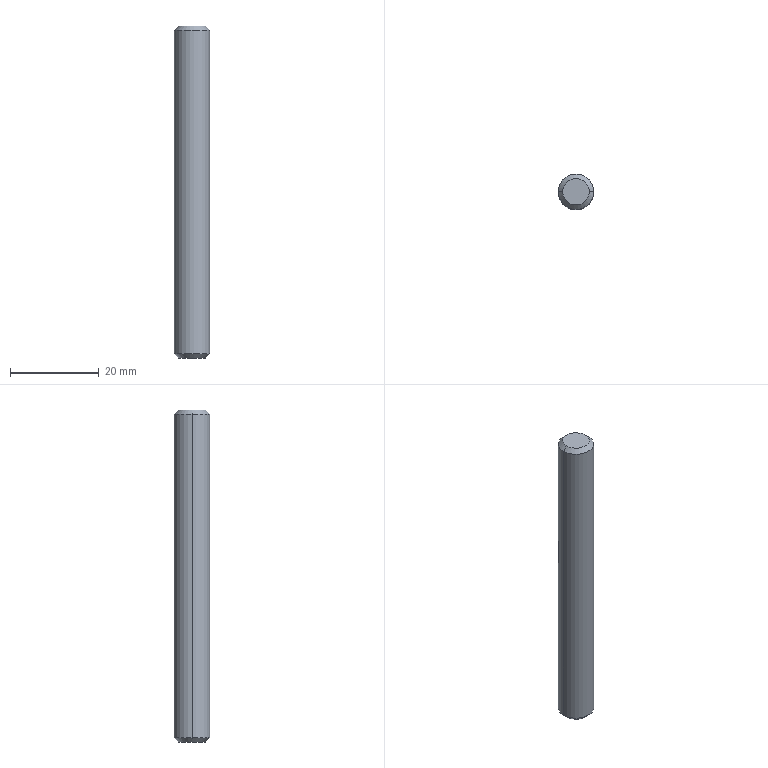Part | STEP file | CHOT DINH VI | 1 solid | 8 faces | box 8 x 8 x 75 mm | volume 3747 mm3 | cone 4 | cylinder 2 | plane 2 | commonest cylinder face diameters 8 x2
STEP:
#1=CARTESIAN_POINT('',(0.,0.,0.));
#2=DIRECTION('',(0.,0.,1.));
#3=DIRECTION('',(1.,0.,0.));
#4=AXIS2_PLACEMENT_3D('',#1,#2,#3);
#5=CARTESIAN_POINT('',(4.,0.,1.));
#6=VERTEX_POINT('',#5);
#7=CARTESIAN_POINT('',(-4.,0.,1.));
#8=VERTEX_POINT('',#7);
#9=CARTESIAN_POINT('',(0.,0.,1.));
#10=DIRECTION('',(0.,0.,1.));
#11=DIRECTION('',(1.,0.,0.));
#12=AXIS2_PLACEMENT_3D('',#9,#10,#11);
#13=CIRCLE('',#12,4.);
#14=CARTESIAN_POINT('',(0.,0.,0.));
#15=DIRECTION('',(0.,0.,1.));
#16=DIRECTION('',(1.,0.,0.));
#17=AXIS2_PLACEMENT_3D('',#14,#15,#16);
#18=CYLINDRICAL_SURFACE('',#17,4.);
#19=CARTESIAN_POINT('',(0.,1.));
#20=DIRECTION('',(1.,0.));
#21=VECTOR('',#20,1.);
#22=LINE('',#19,#21);
#23=(GEOMETRIC_REPRESENTATION_CONTEXT(2)PARAMETRIC_REPRESENTATION_CONTEXT()REPRESENTATION_CONTEXT('',''));
#24=DEFINITIONAL_REPRESENTATION('',(#22),#23);
#25=PCURVE('',#18,#24);
#26=CARTESIAN_POINT('',(0.,0.,1.));
#27=DIRECTION('',(0.,0.,1.));
#28=DIRECTION('',(1.,0.,0.));
#29=AXIS2_PLACEMENT_3D('',#26,#27,#28);
#30=CONICAL_SURFACE('',#29,4.,0.7854);
#31=CARTESIAN_POINT('',(0.,0.));
#32=DIRECTION('',(1.,0.));
#33=VECTOR('',#32,1.);
#34=LINE('',#31,#33);
#35=(GEOMETRIC_REPRESENTATION_CONTEXT(2)PARAMETRIC_REPRESENTATION_CONTEXT()REPRESENTATION_CONTEXT('',''));
#36=DEFINITIONAL_REPRESENTATION('',(#34),#35);
#37=PCURVE('',#30,#36);
#38=SURFACE_CURVE('',#13,(#25,#37),.PCURVE_S1.);
#39=EDGE_CURVE('',#6,#8,#38,.T.);
#40=ORIENTED_EDGE('',*,*,#39,.T.);
#41=CARTESIAN_POINT('',(-4.,0.,74.));
#42=VERTEX_POINT('',#41);
#43=CARTESIAN_POINT('',(-4.,0.,0.));
#44=DIRECTION('',(0.,0.,1.));
#45=VECTOR('',#44,1.);
#46=LINE('',#43,#45);
#47=CARTESIAN_POINT('',(3.142,0.));
#48=DIRECTION('',(0.,1.));
#49=VECTOR('',#48,1.);
#50=LINE('',#47,#49);
#51=(GEOMETRIC_REPRESENTATION_CONTEXT(2)PARAMETRIC_REPRESENTATION_CONTEXT()REPRESENTATION_CONTEXT('',''));
#52=DEFINITIONAL_REPRESENTATION('',(#50),#51);
#53=PCURVE('',#18,#52);
#54=CARTESIAN_POINT('',(0.,0.,0.));
#55=DIRECTION('',(0.,0.,1.));
#56=DIRECTION('',(1.,0.,0.));
#57=AXIS2_PLACEMENT_3D('',#54,#55,#56);
#58=CYLINDRICAL_SURFACE('',#57,4.);
#59=CARTESIAN_POINT('',(3.142,0.));
#60=DIRECTION('',(0.,1.));
#61=VECTOR('',#60,1.);
#62=LINE('',#59,#61);
#63=(GEOMETRIC_REPRESENTATION_CONTEXT(2)PARAMETRIC_REPRESENTATION_CONTEXT()REPRESENTATION_CONTEXT('',''));
#64=DEFINITIONAL_REPRESENTATION('',(#62),#63);
#65=PCURVE('',#58,#64);
#66=SURFACE_CURVE('',#46,(#53,#65),.PCURVE_S1.);
#67=EDGE_CURVE('',#8,#42,#66,.T.);
#68=ORIENTED_EDGE('',*,*,#67,.T.);
#69=CARTESIAN_POINT('',(4.,0.,74.));
#70=VERTEX_POINT('',#69);
#71=CARTESIAN_POINT('',(0.,0.,74.));
#72=DIRECTION('',(0.,0.,-1.));
#73=DIRECTION('',(1.,0.,0.));
#74=AXIS2_PLACEMENT_3D('',#71,#72,#73);
#75=CIRCLE('',#74,4.);
#76=CARTESIAN_POINT('',(6.283,74.));
#77=DIRECTION('',(-1.,0.));
#78=VECTOR('',#77,1.);
#79=LINE('',#76,#78);
#80=(GEOMETRIC_REPRESENTATION_CONTEXT(2)PARAMETRIC_REPRESENTATION_CONTEXT()REPRESENTATION_CONTEXT('',''));
#81=DEFINITIONAL_REPRESENTATION('',(#79),#80);
#82=PCURVE('',#18,#81);
#83=CARTESIAN_POINT('',(0.,0.,74.));
#84=DIRECTION('',(0.,0.,-1.));
#85=DIRECTION('',(-1.,0.,0.));
#86=AXIS2_PLACEMENT_3D('',#83,#84,#85);
#87=CONICAL_SURFACE('',#86,4.,0.7854);
#88=CARTESIAN_POINT('',(-3.142,0.));
#89=DIRECTION('',(1.,0.));
#90=VECTOR('',#89,1.);
#91=LINE('',#88,#90);
#92=(GEOMETRIC_REPRESENTATION_CONTEXT(2)PARAMETRIC_REPRESENTATION_CONTEXT()REPRESENTATION_CONTEXT('',''));
#93=DEFINITIONAL_REPRESENTATION('',(#91),#92);
#94=PCURVE('',#87,#93);
#95=SURFACE_CURVE('',#75,(#82,#94),.PCURVE_S1.);
#96=EDGE_CURVE('',#42,#70,#95,.T.);
#97=ORIENTED_EDGE('',*,*,#96,.T.);
#98=CARTESIAN_POINT('',(4.,0.,0.));
#99=DIRECTION('',(0.,0.,1.));
#100=VECTOR('',#99,1.);
#101=LINE('',#98,#100);
#102=CARTESIAN_POINT('',(0.,0.));
#103=DIRECTION('',(0.,1.));
#104=VECTOR('',#103,1.);
#105=LINE('',#102,#104);
#106=(GEOMETRIC_REPRESENTATION_CONTEXT(2)PARAMETRIC_REPRESENTATION_CONTEXT()REPRESENTATION_CONTEXT('',''));
#107=DEFINITIONAL_REPRESENTATION('',(#105),#106);
#108=PCURVE('',#18,#107);
#109=CARTESIAN_POINT('',(6.283,0.));
#110=DIRECTION('',(0.,1.));
#111=VECTOR('',#110,1.);
#112=LINE('',#109,#111);
#113=(GEOMETRIC_REPRESENTATION_CONTEXT(2)PARAMETRIC_REPRESENTATION_CONTEXT()REPRESENTATION_CONTEXT('',''));
#114=DEFINITIONAL_REPRESENTATION('',(#112),#113);
#115=PCURVE('',#58,#114);
#116=SURFACE_CURVE('',#101,(#108,#115),.PCURVE_S1.);
#117=EDGE_CURVE('',#6,#70,#116,.T.);
#118=ORIENTED_EDGE('',*,*,#117,.F.);
#119=EDGE_LOOP('',(#40,#68,#97,#118));
#120=FACE_BOUND('',#119,.T.);
#121=ADVANCED_FACE('',(#120),#18,.T.);
#122=CARTESIAN_POINT('',(3.,0.,0.));
#123=VERTEX_POINT('',#122);
#124=CARTESIAN_POINT('',(-3.,0.,0.));
#125=VERTEX_POINT('',#124);
#126=CARTESIAN_POINT('',(0.,0.,0.));
#127=DIRECTION('',(0.,0.,1.));
#128=DIRECTION('',(1.,0.,0.));
#129=AXIS2_PLACEMENT_3D('',#126,#127,#128);
#130=CIRCLE('',#129,3.);
#131=CARTESIAN_POINT('',(0.,-1.));
#132=DIRECTION('',(1.,0.));
#133=VECTOR('',#132,1.);
#134=LINE('',#131,#133);
#135=(GEOMETRIC_REPRESENTATION_CONTEXT(2)PARAMETRIC_REPRESENTATION_CONTEXT()REPRESENTATION_CONTEXT('',''));
#136=DEFINITIONAL_REPRESENTATION('',(#134),#135);
#137=PCURVE('',#30,#136);
#138=CARTESIAN_POINT('',(0.,0.,0.));
#139=DIRECTION('',(0.,0.,-1.));
#140=DIRECTION('',(-1.,0.,0.));
#141=AXIS2_PLACEMENT_3D('',#138,#139,#140);
#142=PLANE('',#141);
#143=CARTESIAN_POINT('',(-3.,0.));
#144=CARTESIAN_POINT('',(-3.,5.196));
#145=CARTESIAN_POINT('',(1.5,2.598));
#146=CARTESIAN_POINT('',(6.,0.));
#147=CARTESIAN_POINT('',(1.5,-2.598));
#148=CARTESIAN_POINT('',(-3.,-5.196));
#149=CARTESIAN_POINT('',(-3.,0.));
#150=(BOUNDED_CURVE()B_SPLINE_CURVE(2,(#143,#144,#145,#146,#147,#148,#149),.UNSPECIFIED.,.T.,.F.)B_SPLINE_CURVE_WITH_KNOTS((1,2,2,2,2,1),(-2.094,0.,2.094,4.189,6.283,8.378),.UNSPECIFIED.)CURVE()GEOMETRIC_REPRESENTATION_ITEM()RATIONAL_B_SPLINE_CURVE((1.,0.5,1.,0.5,1.,0.5,1.))REPRESENTATION_ITEM(''));
#151=(GEOMETRIC_REPRESENTATION_CONTEXT(2)PARAMETRIC_REPRESENTATION_CONTEXT()REPRESENTATION_CONTEXT('',''));
#152=DEFINITIONAL_REPRESENTATION('',(#150),#151);
#153=PCURVE('',#142,#152);
#154=SURFACE_CURVE('',#130,(#137,#153),.PCURVE_S1.);
#155=EDGE_CURVE('',#123,#125,#154,.T.);
#156=ORIENTED_EDGE('',*,*,#155,.T.);
#157=CARTESIAN_POINT('',(-4.,0.,1.));
#158=DIRECTION('',(-0.7071,0.,0.7071));
#159=VECTOR('',#158,1.);
#160=LINE('',#157,#159);
#161=CARTESIAN_POINT('',(3.142,0.));
#162=DIRECTION('',(0.,1.));
#163=VECTOR('',#162,1.);
#164=LINE('',#161,#163);
#165=(GEOMETRIC_REPRESENTATION_CONTEXT(2)PARAMETRIC_REPRESENTATION_CONTEXT()REPRESENTATION_CONTEXT('',''));
#166=DEFINITIONAL_REPRESENTATION('',(#164),#165);
#167=PCURVE('',#30,#166);
#168=CARTESIAN_POINT('',(0.,0.,1.));
#169=DIRECTION('',(0.,0.,1.));
#170=DIRECTION('',(1.,0.,0.));
#171=AXIS2_PLACEMENT_3D('',#168,#169,#170);
#172=CONICAL_SURFACE('',#171,4.,0.7854);
#173=CARTESIAN_POINT('',(3.142,0.));
#174=DIRECTION('',(0.,1.));
#175=VECTOR('',#174,1.);
#176=LINE('',#173,#175);
#177=(GEOMETRIC_REPRESENTATION_CONTEXT(2)PARAMETRIC_REPRESENTATION_CONTEXT()REPRESENTATION_CONTEXT('',''));
#178=DEFINITIONAL_REPRESENTATION('',(#176),#177);
#179=PCURVE('',#172,#178);
#180=SURFACE_CURVE('',#160,(#167,#179),.PCURVE_S1.);
#181=EDGE_CURVE('',#125,#8,#180,.T.);
#182=ORIENTED_EDGE('',*,*,#181,.T.);
#183=ORIENTED_EDGE('',*,*,#39,.F.);
#184=CARTESIAN_POINT('',(4.,0.,1.));
#185=DIRECTION('',(0.7071,0.,0.7071));
#186=VECTOR('',#185,1.);
#187=LINE('',#184,#186);
#188=CARTESIAN_POINT('',(0.,0.));
#189=DIRECTION('',(0.,1.));
#190=VECTOR('',#189,1.);
#191=LINE('',#188,#190);
#192=(GEOMETRIC_REPRESENTATION_CONTEXT(2)PARAMETRIC_REPRESENTATION_CONTEXT()REPRESENTATION_CONTEXT('',''));
#193=DEFINITIONAL_REPRESENTATION('',(#191),#192);
#194=PCURVE('',#30,#193);
#195=CARTESIAN_POINT('',(6.283,0.));
#196=DIRECTION('',(0.,1.));
#197=VECTOR('',#196,1.);
#198=LINE('',#195,#197);
#199=(GEOMETRIC_REPRESENTATION_CONTEXT(2)PARAMETRIC_REPRESENTATION_CONTEXT()REPRESENTATION_CONTEXT('',''));
#200=DEFINITIONAL_REPRESENTATION('',(#198),#199);
#201=PCURVE('',#172,#200);
#202=SURFACE_CURVE('',#187,(#194,#201),.PCURVE_S1.);
#203=EDGE_CURVE('',#123,#6,#202,.T.);
#204=ORIENTED_EDGE('',*,*,#203,.F.);
#205=EDGE_LOOP('',(#156,#182,#183,#204));
#206=FACE_BOUND('',#205,.T.);
#207=ADVANCED_FACE('',(#206),#30,.T.);
#208=CARTESIAN_POINT('',(-3.,0.,75.));
#209=VERTEX_POINT('',#208);
#210=CARTESIAN_POINT('',(3.,0.,75.));
#211=VERTEX_POINT('',#210);
#212=CARTESIAN_POINT('',(0.,0.,75.));
#213=DIRECTION('',(0.,0.,-1.));
#214=DIRECTION('',(-1.,0.,0.));
#215=AXIS2_PLACEMENT_3D('',#212,#213,#214);
#216=CIRCLE('',#215,3.);
#217=CARTESIAN_POINT('',(0.,-1.));
#218=DIRECTION('',(1.,0.));
#219=VECTOR('',#218,1.);
#220=LINE('',#217,#219);
#221=(GEOMETRIC_REPRESENTATION_CONTEXT(2)PARAMETRIC_REPRESENTATION_CONTEXT()REPRESENTATION_CONTEXT('',''));
#222=DEFINITIONAL_REPRESENTATION('',(#220),#221);
#223=PCURVE('',#87,#222);
#224=CARTESIAN_POINT('',(0.,0.,75.));
#225=DIRECTION('',(0.,0.,-1.));
#226=DIRECTION('',(-1.,0.,0.));
#227=AXIS2_PLACEMENT_3D('',#224,#225,#226);
#228=PLANE('',#227);
#229=CARTESIAN_POINT('',(0.,0.));
#230=DIRECTION('',(1.,0.));
#231=AXIS2_PLACEMENT_2D('',#229,#230);
#232=CIRCLE('',#231,3.);
#233=(GEOMETRIC_REPRESENTATION_CONTEXT(2)PARAMETRIC_REPRESENTATION_CONTEXT()REPRESENTATION_CONTEXT('',''));
#234=DEFINITIONAL_REPRESENTATION('',(#232),#233);
#235=PCURVE('',#228,#234);
#236=SURFACE_CURVE('',#216,(#223,#235),.PCURVE_S1.);
#237=EDGE_CURVE('',#209,#211,#236,.T.);
#238=ORIENTED_EDGE('',*,*,#237,.T.);
#239=CARTESIAN_POINT('',(4.,0.,74.));
#240=DIRECTION('',(0.7071,0.,-0.7071));
#241=VECTOR('',#240,1.);
#242=LINE('',#239,#241);
#243=CARTESIAN_POINT('',(3.142,0.));
#244=DIRECTION('',(0.,1.));
#245=VECTOR('',#244,1.);
#246=LINE('',#243,#245);
#247=(GEOMETRIC_REPRESENTATION_CONTEXT(2)PARAMETRIC_REPRESENTATION_CONTEXT()REPRESENTATION_CONTEXT('',''));
#248=DEFINITIONAL_REPRESENTATION('',(#246),#247);
#249=PCURVE('',#87,#248);
#250=CARTESIAN_POINT('',(0.,0.,74.));
#251=DIRECTION('',(0.,0.,-1.));
#252=DIRECTION('',(-1.,0.,0.));
#253=AXIS2_PLACEMENT_3D('',#250,#251,#252);
#254=CONICAL_SURFACE('',#253,4.,0.7854);
#255=CARTESIAN_POINT('',(3.142,0.));
#256=DIRECTION('',(0.,1.));
#257=VECTOR('',#256,1.);
#258=LINE('',#255,#257);
#259=(GEOMETRIC_REPRESENTATION_CONTEXT(2)PARAMETRIC_REPRESENTATION_CONTEXT()REPRESENTATION_CONTEXT('',''));
#260=DEFINITIONAL_REPRESENTATION('',(#258),#259);
#261=PCURVE('',#254,#260);
#262=SURFACE_CURVE('',#242,(#249,#261),.PCURVE_S1.);
#263=EDGE_CURVE('',#211,#70,#262,.T.);
#264=ORIENTED_EDGE('',*,*,#263,.T.);
#265=ORIENTED_EDGE('',*,*,#96,.F.);
#266=CARTESIAN_POINT('',(-4.,0.,74.));
#267=DIRECTION('',(-0.7071,0.,-0.7071));
#268=VECTOR('',#267,1.);
#269=LINE('',#266,#268);
#270=CARTESIAN_POINT('',(0.,0.));
#271=DIRECTION('',(0.,1.));
#272=VECTOR('',#271,1.);
#273=LINE('',#270,#272);
#274=(GEOMETRIC_REPRESENTATION_CONTEXT(2)PARAMETRIC_REPRESENTATION_CONTEXT()REPRESENTATION_CONTEXT('',''));
#275=DEFINITIONAL_REPRESENTATION('',(#273),#274);
#276=PCURVE('',#87,#275);
#277=CARTESIAN_POINT('',(6.283,0.));
#278=DIRECTION('',(0.,1.));
#279=VECTOR('',#278,1.);
#280=LINE('',#277,#279);
#281=(GEOMETRIC_REPRESENTATION_CONTEXT(2)PARAMETRIC_REPRESENTATION_CONTEXT()REPRESENTATION_CONTEXT('',''));
#282=DEFINITIONAL_REPRESENTATION('',(#280),#281);
#283=PCURVE('',#254,#282);
#284=SURFACE_CURVE('',#269,(#276,#283),.PCURVE_S1.);
#285=EDGE_CURVE('',#209,#42,#284,.T.);
#286=ORIENTED_EDGE('',*,*,#285,.F.);
#287=EDGE_LOOP('',(#238,#264,#265,#286));
#288=FACE_BOUND('',#287,.T.);
#289=ADVANCED_FACE('',(#288),#87,.T.);
#290=ORIENTED_EDGE('',*,*,#67,.F.);
#291=CARTESIAN_POINT('',(0.,0.,1.));
#292=DIRECTION('',(0.,0.,1.));
#293=DIRECTION('',(1.,0.,0.));
#294=AXIS2_PLACEMENT_3D('',#291,#292,#293);
#295=CIRCLE('',#294,4.);
#296=CARTESIAN_POINT('',(0.,1.));
#297=DIRECTION('',(1.,0.));
#298=VECTOR('',#297,1.);
#299=LINE('',#296,#298);
#300=(GEOMETRIC_REPRESENTATION_CONTEXT(2)PARAMETRIC_REPRESENTATION_CONTEXT()REPRESENTATION_CONTEXT('',''));
#301=DEFINITIONAL_REPRESENTATION('',(#299),#300);
#302=PCURVE('',#58,#301);
#303=CARTESIAN_POINT('',(0.,0.));
#304=DIRECTION('',(1.,0.));
#305=VECTOR('',#304,1.);
#306=LINE('',#303,#305);
#307=(GEOMETRIC_REPRESENTATION_CONTEXT(2)PARAMETRIC_REPRESENTATION_CONTEXT()REPRESENTATION_CONTEXT('',''));
#308=DEFINITIONAL_REPRESENTATION('',(#306),#307);
#309=PCURVE('',#172,#308);
#310=SURFACE_CURVE('',#295,(#302,#309),.PCURVE_S1.);
#311=EDGE_CURVE('',#8,#6,#310,.T.);
#312=ORIENTED_EDGE('',*,*,#311,.T.);
#313=ORIENTED_EDGE('',*,*,#117,.T.);
#314=CARTESIAN_POINT('',(0.,0.,74.));
#315=DIRECTION('',(0.,0.,-1.));
#316=DIRECTION('',(1.,0.,0.));
#317=AXIS2_PLACEMENT_3D('',#314,#315,#316);
#318=CIRCLE('',#317,4.);
#319=CARTESIAN_POINT('',(6.283,74.));
#320=DIRECTION('',(-1.,0.));
#321=VECTOR('',#320,1.);
#322=LINE('',#319,#321);
#323=(GEOMETRIC_REPRESENTATION_CONTEXT(2)PARAMETRIC_REPRESENTATION_CONTEXT()REPRESENTATION_CONTEXT('',''));
#324=DEFINITIONAL_REPRESENTATION('',(#322),#323);
#325=PCURVE('',#58,#324);
#326=CARTESIAN_POINT('',(3.142,0.));
#327=DIRECTION('',(1.,0.));
#328=VECTOR('',#327,1.);
#329=LINE('',#326,#328);
#330=(GEOMETRIC_REPRESENTATION_CONTEXT(2)PARAMETRIC_REPRESENTATION_CONTEXT()REPRESENTATION_CONTEXT('',''));
#331=DEFINITIONAL_REPRESENTATION('',(#329),#330);
#332=PCURVE('',#254,#331);
#333=SURFACE_CURVE('',#318,(#325,#332),.PCURVE_S1.);
#334=EDGE_CURVE('',#70,#42,#333,.T.);
#335=ORIENTED_EDGE('',*,*,#334,.T.);
#336=EDGE_LOOP('',(#290,#312,#313,#335));
#337=FACE_BOUND('',#336,.T.);
#338=ADVANCED_FACE('',(#337),#58,.T.);
#339=ORIENTED_EDGE('',*,*,#181,.F.);
#340=CARTESIAN_POINT('',(0.,0.,0.));
#341=DIRECTION('',(0.,0.,1.));
#342=DIRECTION('',(1.,0.,0.));
#343=AXIS2_PLACEMENT_3D('',#340,#341,#342);
#344=CIRCLE('',#343,3.);
#345=CARTESIAN_POINT('',(0.,-1.));
#346=DIRECTION('',(1.,0.));
#347=VECTOR('',#346,1.);
#348=LINE('',#345,#347);
#349=(GEOMETRIC_REPRESENTATION_CONTEXT(2)PARAMETRIC_REPRESENTATION_CONTEXT()REPRESENTATION_CONTEXT('',''));
#350=DEFINITIONAL_REPRESENTATION('',(#348),#349);
#351=PCURVE('',#172,#350);
#352=CARTESIAN_POINT('',(-3.,0.));
#353=CARTESIAN_POINT('',(-3.,5.196));
#354=CARTESIAN_POINT('',(1.5,2.598));
#355=CARTESIAN_POINT('',(6.,0.));
#356=CARTESIAN_POINT('',(1.5,-2.598));
#357=CARTESIAN_POINT('',(-3.,-5.196));
#358=CARTESIAN_POINT('',(-3.,0.));
#359=(BOUNDED_CURVE()B_SPLINE_CURVE(2,(#352,#353,#354,#355,#356,#357,#358),.UNSPECIFIED.,.T.,.F.)B_SPLINE_CURVE_WITH_KNOTS((1,2,2,2,2,1),(-2.094,0.,2.094,4.189,6.283,8.378),.UNSPECIFIED.)CURVE()GEOMETRIC_REPRESENTATION_ITEM()RATIONAL_B_SPLINE_CURVE((1.,0.5,1.,0.5,1.,0.5,1.))REPRESENTATION_ITEM(''));
#360=(GEOMETRIC_REPRESENTATION_CONTEXT(2)PARAMETRIC_REPRESENTATION_CONTEXT()REPRESENTATION_CONTEXT('',''));
#361=DEFINITIONAL_REPRESENTATION('',(#359),#360);
#362=PCURVE('',#142,#361);
#363=SURFACE_CURVE('',#344,(#351,#362),.PCURVE_S1.);
#364=EDGE_CURVE('',#125,#123,#363,.T.);
#365=ORIENTED_EDGE('',*,*,#364,.T.);
#366=ORIENTED_EDGE('',*,*,#203,.T.);
#367=ORIENTED_EDGE('',*,*,#311,.F.);
#368=EDGE_LOOP('',(#339,#365,#366,#367));
#369=FACE_BOUND('',#368,.T.);
#370=ADVANCED_FACE('',(#369),#172,.T.);
#371=ORIENTED_EDGE('',*,*,#263,.F.);
#372=CARTESIAN_POINT('',(0.,0.,75.));
#373=DIRECTION('',(0.,0.,-1.));
#374=DIRECTION('',(-1.,0.,0.));
#375=AXIS2_PLACEMENT_3D('',#372,#373,#374);
#376=CIRCLE('',#375,3.);
#377=CARTESIAN_POINT('',(0.,-1.));
#378=DIRECTION('',(1.,0.));
#379=VECTOR('',#378,1.);
#380=LINE('',#377,#379);
#381=(GEOMETRIC_REPRESENTATION_CONTEXT(2)PARAMETRIC_REPRESENTATION_CONTEXT()REPRESENTATION_CONTEXT('',''));
#382=DEFINITIONAL_REPRESENTATION('',(#380),#381);
#383=PCURVE('',#254,#382);
#384=CARTESIAN_POINT('',(0.,0.));
#385=DIRECTION('',(1.,0.));
#386=AXIS2_PLACEMENT_2D('',#384,#385);
#387=CIRCLE('',#386,3.);
#388=(GEOMETRIC_REPRESENTATION_CONTEXT(2)PARAMETRIC_REPRESENTATION_CONTEXT()REPRESENTATION_CONTEXT('',''));
#389=DEFINITIONAL_REPRESENTATION('',(#387),#388);
#390=PCURVE('',#228,#389);
#391=SURFACE_CURVE('',#376,(#383,#390),.PCURVE_S1.);
#392=EDGE_CURVE('',#211,#209,#391,.T.);
#393=ORIENTED_EDGE('',*,*,#392,.T.);
#394=ORIENTED_EDGE('',*,*,#285,.T.);
#395=ORIENTED_EDGE('',*,*,#334,.F.);
#396=EDGE_LOOP('',(#371,#393,#394,#395));
#397=FACE_BOUND('',#396,.T.);
#398=ADVANCED_FACE('',(#397),#254,.T.);
#399=ORIENTED_EDGE('',*,*,#155,.F.);
#400=ORIENTED_EDGE('',*,*,#364,.F.);
#401=EDGE_LOOP('',(#399,#400));
#402=FACE_BOUND('',#401,.T.);
#403=ADVANCED_FACE('',(#402),#142,.T.);
#404=ORIENTED_EDGE('',*,*,#237,.F.);
#405=ORIENTED_EDGE('',*,*,#392,.F.);
#406=EDGE_LOOP('',(#404,#405));
#407=FACE_BOUND('',#406,.T.);
#408=ADVANCED_FACE('',(#407),#228,.F.);
#409=CLOSED_SHELL('',(#121,#207,#289,#338,#370,#398,#403,#408));
#410=MANIFOLD_SOLID_BREP('',#409);
#411=(LENGTH_UNIT()NAMED_UNIT(*)SI_UNIT(.MILLI.,.METRE.));
#412=UNCERTAINTY_MEASURE_WITH_UNIT(LENGTH_MEASURE(0.0000001),#411,'','');
#413=(NAMED_UNIT(*)PLANE_ANGLE_UNIT()SI_UNIT($,.RADIAN.));
#414=(NAMED_UNIT(*)SI_UNIT($,.STERADIAN.)SOLID_ANGLE_UNIT());
#415=(GEOMETRIC_REPRESENTATION_CONTEXT(3)GLOBAL_UNCERTAINTY_ASSIGNED_CONTEXT((#412))GLOBAL_UNIT_ASSIGNED_CONTEXT((#411,#413,#414))REPRESENTATION_CONTEXT('',''));
#416=ADVANCED_BREP_SHAPE_REPRESENTATION('',(#4,#410),#415);